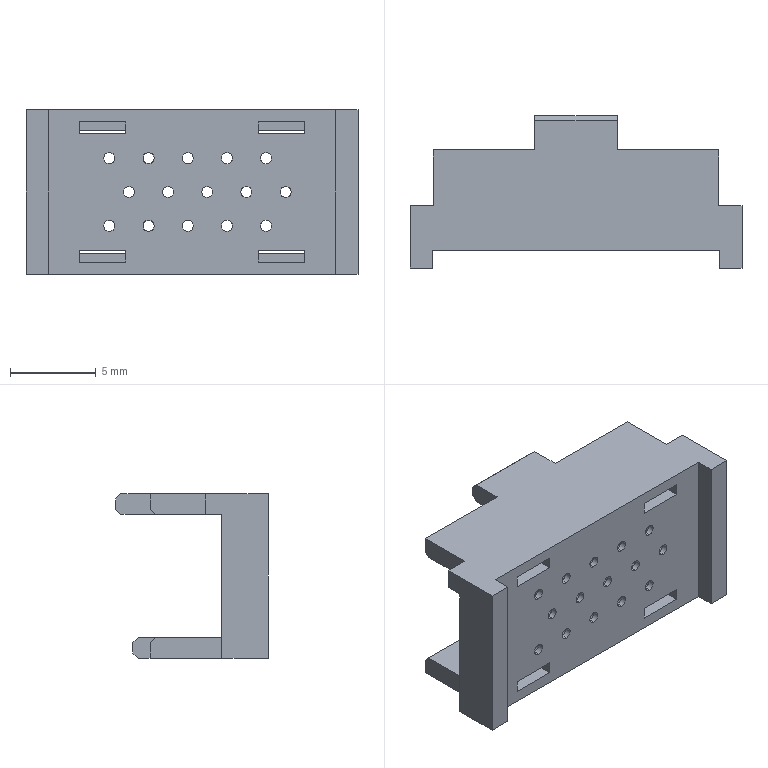Part | STEP file | COVER | 1 solid | 214 faces | box 19.4 x 8.9 x 9.6 mm | volume 433.37 mm3 | plane 184 | cylinder 30 | commonest cylinder face diameters 0.65 x30